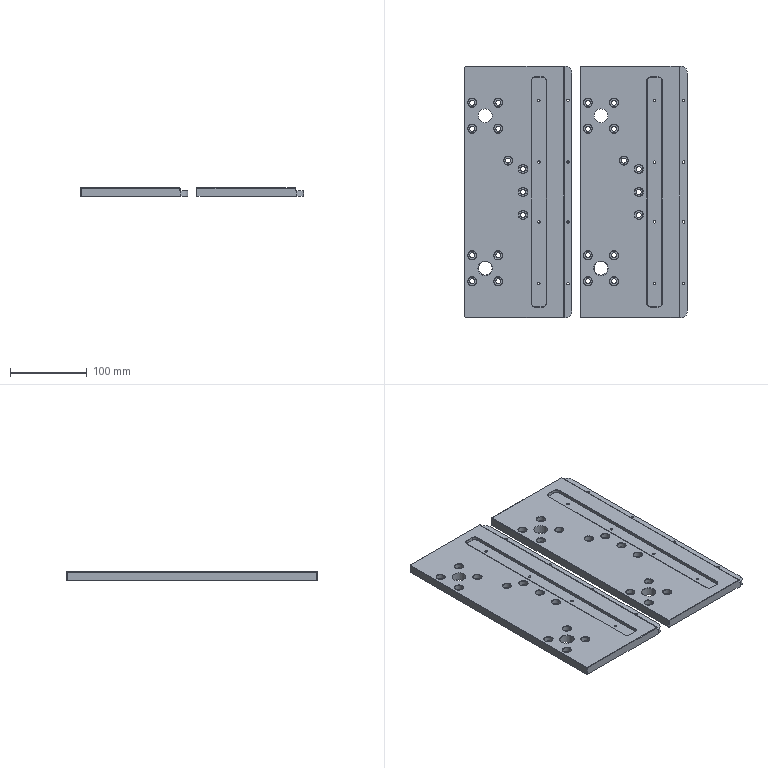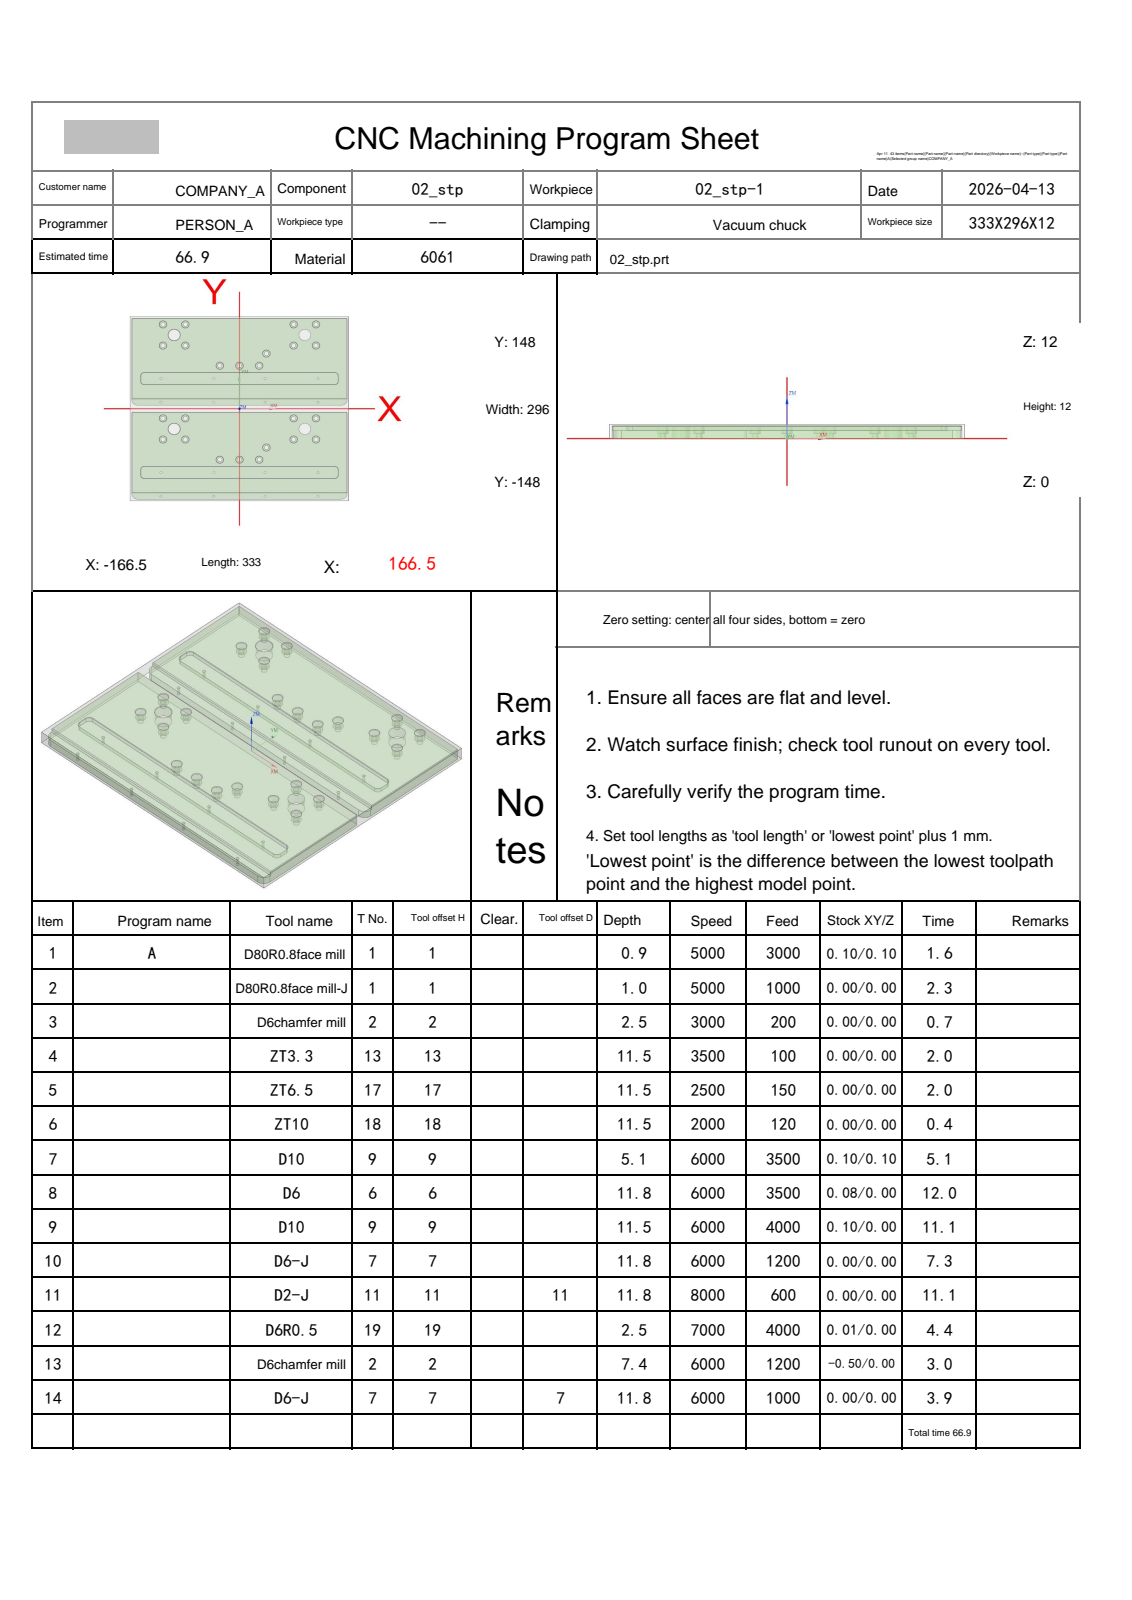NC program | NX | posted by the shop | part box 291 x 328 x 11 mm
Lines 616 to 1679 of 9762:
N8 T06 M06
(D6  D=6. R=0. H=06 ce=0.10 di=0.10)
G00 G90 G54 X-37.711 Y-143.4 M03 S6000
G43 H06 Z31.
M08
Z11.5
G01 X0.0 Z10.513 F3500.
X155.
G03 X159.957 Y-141.3 I0.0 J6.9
G01 X-159.957
G03 X-155. Y-143.4 I4.957 J4.8
G01 X0.0
Y-146.1
X155.
G03 X164.367 Y-138.6 I0.0 J9.6
G01 X-164.367
G03 X-155. Y-146.1 I9.367 J2.1
G01 X0.0
X.5
Z11.013
G00 Z11.5
X-37.711 Y-143.4
Z11.013
G01 X0.0 Z10.025
X155.
G03 X159.957 Y-141.3 I0.0 J6.9
G01 X-159.957
G03 X-155. Y-143.4 I4.957 J4.8
G01 X0.0
Y-146.1
X155.
G03 X164.367 Y-138.6 I0.0 J9.6
G01 X-164.367
G03 X-155. Y-146.1 I9.367 J2.1
G01 X0.0
X.5
Z10.525
G00 Z11.013
X-37.711 Y-143.4
Z10.525
G01 X0.0 Z9.538
X155.
G03 X159.957 Y-141.3 I0.0 J6.9
G01 X-159.957
G03 X-155. Y-143.4 I4.957 J4.8
G01 X0.0
Y-146.1
X155.
G03 X164.367 Y-138.6 I0.0 J9.6
G01 X-164.367
G03 X-155. Y-146.1 I9.367 J2.1
G01 X0.0
X.5
Z10.038
G00 Z10.525
X-37.711 Y-143.4
Z10.038
G01 X0.0 Z9.05
X155.
G03 X159.957 Y-141.3 I0.0 J6.9
G01 X-159.957
G03 X-155. Y-143.4 I4.957 J4.8
G01 X0.0
Y-146.1
X155.
G03 X164.367 Y-138.6 I0.0 J9.6
G01 X-164.367
G03 X-155. Y-146.1 I9.367 J2.1
G01 X0.0
X.5
Z9.55
G00 Z10.038
X-37.711 Y-143.4
Z9.55
G01 X0.0 Z8.563
X155.
G03 X159.957 Y-141.3 I0.0 J6.9
G01 X-159.957
G03 X-155. Y-143.4 I4.957 J4.8
G01 X0.0
Y-146.1
X155.
G03 X164.367 Y-138.6 I0.0 J9.6
G01 X-164.367
G03 X-155. Y-146.1 I9.367 J2.1
G01 X0.0
X.5
Z9.063
G00 Z9.55
X-37.711 Y-143.4
Z9.063
G01 X0.0 Z8.075
X155.
G03 X159.957 Y-141.3 I0.0 J6.9
G01 X-159.957
G03 X-155. Y-143.4 I4.957 J4.8
G01 X0.0
Y-146.1
X155.
G03 X164.367 Y-138.6 I0.0 J9.6
G01 X-164.367
G03 X-155. Y-146.1 I9.367 J2.1
G01 X0.0
X.5
Z8.575
G00 Z9.063
X-37.711 Y-143.4
Z8.575
G01 X0.0 Z7.588
X155.
G03 X159.957 Y-141.3 I0.0 J6.9
G01 X-159.957
G03 X-155. Y-143.4 I4.957 J4.8
G01 X0.0
Y-146.1
X155.
G03 X164.367 Y-138.6 I0.0 J9.6
G01 X-164.367
G03 X-155. Y-146.1 I9.367 J2.1
G01 X0.0
X.5
Z8.088
G00 Z8.575
X-37.711 Y-143.4
Z8.088
G01 X0.0 Z7.1
X155.
G03 X159.957 Y-141.3 I0.0 J6.9
G01 X-159.957
G03 X-155. Y-143.4 I4.957 J4.8
G01 X0.0
Y-146.1
X155.
G03 X164.367 Y-138.6 I0.0 J9.6
G01 X-164.367
G03 X-155. Y-146.1 I9.367 J2.1
G01 X0.0
X.5
Z7.6
G00 Z31.
X-37.711 Y7.6
Z11.5
G01 X0.0 Z10.513
X155.
G03 X159.957 Y9.7 I0.0 J6.9
G01 X-159.957
G03 X-155. Y7.6 I4.957 J4.8
G01 X0.0
Y4.9
X155.
G03 X164.367 Y12.4 I0.0 J9.6
G01 X-164.367
G03 X-155. Y4.9 I9.367 J2.1
G01 X0.0
X.5
Z11.013
G00 Z11.5
X-37.711 Y7.6
Z11.013
G01 X0.0 Z10.025
X155.
G03 X159.957 Y9.7 I0.0 J6.9
G01 X-159.957
G03 X-155. Y7.6 I4.957 J4.8
G01 X0.0
Y4.9
X155.
G03 X164.367 Y12.4 I0.0 J9.6
G01 X-164.367
G03 X-155. Y4.9 I9.367 J2.1
G01 X0.0
X.5
Z10.525
G00 Z11.013
X-37.711 Y7.6
Z10.525
G01 X0.0 Z9.538
X155.
G03 X159.957 Y9.7 I0.0 J6.9
G01 X-159.957
G03 X-155. Y7.6 I4.957 J4.8
G01 X0.0
Y4.9
X155.
G03 X164.367 Y12.4 I0.0 J9.6
G01 X-164.367
G03 X-155. Y4.9 I9.367 J2.1
G01 X0.0
X.5
Z10.038
G00 Z10.525
X-37.711 Y7.6
Z10.038
G01 X0.0 Z9.05
X155.
G03 X159.957 Y9.7 I0.0 J6.9
G01 X-159.957
G03 X-155. Y7.6 I4.957 J4.8
G01 X0.0
Y4.9
X155.
G03 X164.367 Y12.4 I0.0 J9.6
G01 X-164.367
G03 X-155. Y4.9 I9.367 J2.1
G01 X0.0
X.5
Z9.55
G00 Z10.038
X-37.711 Y7.6
Z9.55
G01 X0.0 Z8.563
X155.
G03 X159.957 Y9.7 I0.0 J6.9
G01 X-159.957
G03 X-155. Y7.6 I4.957 J4.8
G01 X0.0
Y4.9
X155.
G03 X164.367 Y12.4 I0.0 J9.6
G01 X-164.367
G03 X-155. Y4.9 I9.367 J2.1
G01 X0.0
X.5
Z9.063
G00 Z9.55
X-37.711 Y7.6
Z9.063
G01 X0.0 Z8.075
X155.
G03 X159.957 Y9.7 I0.0 J6.9
G01 X-159.957
G03 X-155. Y7.6 I4.957 J4.8
G01 X0.0
Y4.9
X155.
G03 X164.367 Y12.4 I0.0 J9.6
G01 X-164.367
G03 X-155. Y4.9 I9.367 J2.1
G01 X0.0
X.5
Z8.575
G00 Z9.063
X-37.711 Y7.6
Z8.575
G01 X0.0 Z7.588
X155.
G03 X159.957 Y9.7 I0.0 J6.9
G01 X-159.957
G03 X-155. Y7.6 I4.957 J4.8
G01 X0.0
Y4.9
X155.
G03 X164.367 Y12.4 I0.0 J9.6
G01 X-164.367
G03 X-155. Y4.9 I9.367 J2.1
G01 X0.0
X.5
Z8.088
G00 Z8.575
X-37.711 Y7.6
Z8.088
G01 X0.0 Z7.1
X155.
G03 X159.957 Y9.7 I0.0 J6.9
G01 X-159.957
G03 X-155. Y7.6 I4.957 J4.8
G01 X0.0
Y4.9
X155.
G03 X164.367 Y12.4 I0.0 J9.6
G01 X-164.367
G03 X-155. Y4.9 I9.367 J2.1
G01 X0.0
X.5
Z7.6
G00 Z31.
G00 G90 X41. Y-62.4 M03 S6000
Z31.
Z11.8
G41 D06
G01 X40.9 Y-62.408 F2000.
G03 X39.802 Y-63.602 I.1 J-1.194
X41. Y-64.8 I1.198 J0.0
X41. Y-64.8 Z11.3 I0.0 J2.4
X41. Y-64.8 Z10.8 I0.0 J2.4
X41. Y-64.8 Z10.3 I0.0 J2.4
X41. Y-64.8 Z9.8 I0.0 J2.4
X41. Y-64.8 Z9.3 I0.0 J2.4
X41. Y-64.8 Z8.8 I0.0 J2.4
X41. Y-64.8 Z8.3 I0.0 J2.4
X41. Y-64.8 Z7.8 I0.0 J2.4
X41. Y-64.8 Z7.3 I0.0 J2.4
X41. Y-64.8 Z6.8 I0.0 J2.4
X41. Y-64.8 Z6.3 I0.0 J2.4
X41. Y-64.8 Z5.8 I0.0 J2.4
X41. Y-64.8 Z5.3 I0.0 J2.4
X41. Y-64.8 Z4.8 I0.0 J2.4
X39.589 Y-60.458 Z4.5 I0.0 J2.4
X38.6 Y-62.4 I1.411 J-1.942
X41. Y-64.8 I2.4 J0.0
X43.4 Y-62.4 I0.0 J2.4
X41. Y-60. I-2.4 J0.0
X39.589 Y-60.458 I0.0 J-2.4
X39.096 Y-61.427 I.704 J-.969
X40.293 Y-62.625 I1.198 J0.0
X40.914 Y-62.452 I0.0 J1.198
G01 G40 X41. Y-62.4
G00 Z31.
X82.5 Y-15.5
Z11.8
G41 D06
G01 X82.4 Y-15.508
G03 X81.302 Y-16.702 I.1 J-1.194
X82.5 Y-17.9 I1.198 J0.0
X82.5 Y-17.9 Z11.3 I0.0 J2.4
X82.5 Y-17.9 Z10.8 I0.0 J2.4
X82.5 Y-17.9 Z10.3 I0.0 J2.4
X82.5 Y-17.9 Z9.8 I0.0 J2.4
X82.5 Y-17.9 Z9.3 I0.0 J2.4
X82.5 Y-17.9 Z8.8 I0.0 J2.4
X82.5 Y-17.9 Z8.3 I0.0 J2.4
X82.5 Y-17.9 Z7.8 I0.0 J2.4
X82.5 Y-17.9 Z7.3 I0.0 J2.4
X82.5 Y-17.9 Z6.8 I0.0 J2.4
X82.5 Y-17.9 Z6.3 I0.0 J2.4
X82.5 Y-17.9 Z5.8 I0.0 J2.4
X82.5 Y-17.9 Z5.3 I0.0 J2.4
X82.5 Y-17.9 Z4.8 I0.0 J2.4
X81.089 Y-13.558 Z4.5 I0.0 J2.4
X80.1 Y-15.5 I1.411 J-1.942
X82.5 Y-17.9 I2.4 J0.0
X84.9 Y-15.5 I0.0 J2.4
X82.5 Y-13.1 I-2.4 J0.0
X81.089 Y-13.558 I0.0 J-2.4
X80.596 Y-14.527 I.704 J-.969
X81.793 Y-15.725 I1.198 J0.0
X82.414 Y-15.552 I0.0 J1.198
G01 G40 X82.5 Y-15.5
G00 Z31.
X116.5
Z11.8
G41 D06
G01 X116.4 Y-15.508
G03 X115.302 Y-16.702 I.1 J-1.194
X116.5 Y-17.9 I1.198 J0.0
X116.5 Y-17.9 Z11.3 I0.0 J2.4
X116.5 Y-17.9 Z10.8 I0.0 J2.4
X116.5 Y-17.9 Z10.3 I0.0 J2.4
X116.5 Y-17.9 Z9.8 I0.0 J2.4
X116.5 Y-17.9 Z9.3 I0.0 J2.4
X116.5 Y-17.9 Z8.8 I0.0 J2.4
X116.5 Y-17.9 Z8.3 I0.0 J2.4
X116.5 Y-17.9 Z7.8 I0.0 J2.4
X116.5 Y-17.9 Z7.3 I0.0 J2.4
X116.5 Y-17.9 Z6.8 I0.0 J2.4
X116.5 Y-17.9 Z6.3 I0.0 J2.4
X116.5 Y-17.9 Z5.8 I0.0 J2.4
X116.5 Y-17.9 Z5.3 I0.0 J2.4
X116.5 Y-17.9 Z4.8 I0.0 J2.4
X115.089 Y-13.558 Z4.5 I0.0 J2.4
X114.1 Y-15.5 I1.411 J-1.942
X116.5 Y-17.9 I2.4 J0.0
X118.9 Y-15.5 I0.0 J2.4
X116.5 Y-13.1 I-2.4 J0.0
X115.089 Y-13.558 I0.0 J-2.4
X114.596 Y-14.527 I.704 J-.969
X115.793 Y-15.725 I1.198 J0.0
X116.414 Y-15.552 I0.0 J1.198
G01 G40 X116.5 Y-15.5
G00 Z31.
Y-49.5
Z11.8
G41 D06
G01 X116.4 Y-49.508
G03 X115.302 Y-50.702 I.1 J-1.194
X116.5 Y-51.9 I1.198 J0.0
X116.5 Y-51.9 Z11.3 I0.0 J2.4
X116.5 Y-51.9 Z10.8 I0.0 J2.4
X116.5 Y-51.9 Z10.3 I0.0 J2.4
X116.5 Y-51.9 Z9.8 I0.0 J2.4
X116.5 Y-51.9 Z9.3 I0.0 J2.4
X116.5 Y-51.9 Z8.8 I0.0 J2.4
X116.5 Y-51.9 Z8.3 I0.0 J2.4
X116.5 Y-51.9 Z7.8 I0.0 J2.4
X116.5 Y-51.9 Z7.3 I0.0 J2.4
X116.5 Y-51.9 Z6.8 I0.0 J2.4
X116.5 Y-51.9 Z6.3 I0.0 J2.4
X116.5 Y-51.9 Z5.8 I0.0 J2.4
X116.5 Y-51.9 Z5.3 I0.0 J2.4
X116.5 Y-51.9 Z4.8 I0.0 J2.4
X115.089 Y-47.558 Z4.5 I0.0 J2.4
X114.1 Y-49.5 I1.411 J-1.942
X116.5 Y-51.9 I2.4 J0.0
X118.9 Y-49.5 I0.0 J2.4
X116.5 Y-47.1 I-2.4 J0.0
X115.089 Y-47.558 I0.0 J-2.4
X114.596 Y-48.527 I.704 J-.969
X115.793 Y-49.725 I1.198 J0.0
X116.414 Y-49.552 I0.0 J1.198
G01 G40 X116.5 Y-49.5
G00 Z31.
X82.5
Z11.8
G41 D06
G01 X82.4 Y-49.508
G03 X81.302 Y-50.702 I.1 J-1.194
X82.5 Y-51.9 I1.198 J0.0
X82.5 Y-51.9 Z11.3 I0.0 J2.4
X82.5 Y-51.9 Z10.8 I0.0 J2.4
X82.5 Y-51.9 Z10.3 I0.0 J2.4
X82.5 Y-51.9 Z9.8 I0.0 J2.4
X82.5 Y-51.9 Z9.3 I0.0 J2.4
X82.5 Y-51.9 Z8.8 I0.0 J2.4
X82.5 Y-51.9 Z8.3 I0.0 J2.4
X82.5 Y-51.9 Z7.8 I0.0 J2.4
X82.5 Y-51.9 Z7.3 I0.0 J2.4
X82.5 Y-51.9 Z6.8 I0.0 J2.4
X82.5 Y-51.9 Z6.3 I0.0 J2.4
X82.5 Y-51.9 Z5.8 I0.0 J2.4
X82.5 Y-51.9 Z5.3 I0.0 J2.4
X82.5 Y-51.9 Z4.8 I0.0 J2.4
X81.089 Y-47.558 Z4.5 I0.0 J2.4
X80.1 Y-49.5 I1.411 J-1.942
X82.5 Y-51.9 I2.4 J0.0
X84.9 Y-49.5 I0.0 J2.4
X82.5 Y-47.1 I-2.4 J0.0
X81.089 Y-47.558 I0.0 J-2.4
X80.596 Y-48.527 I.704 J-.969
X81.793 Y-49.725 I1.198 J0.0
X82.414 Y-49.552 I0.0 J1.198
G01 G40 X82.5 Y-49.5
G00 Z31.
X30.05 Y-81.9
Z11.8
G41 D06
G01 X29.95 Y-81.908
G03 X28.852 Y-83.102 I.1 J-1.194
X30.05 Y-84.3 I1.198 J0.0
X30.05 Y-84.3 Z11.3 I0.0 J2.4
X30.05 Y-84.3 Z10.8 I0.0 J2.4
X30.05 Y-84.3 Z10.3 I0.0 J2.4
X30.05 Y-84.3 Z9.8 I0.0 J2.4
X30.05 Y-84.3 Z9.3 I0.0 J2.4
X30.05 Y-84.3 Z8.8 I0.0 J2.4
X30.05 Y-84.3 Z8.3 I0.0 J2.4
X30.05 Y-84.3 Z7.8 I0.0 J2.4
X30.05 Y-84.3 Z7.3 I0.0 J2.4
X30.05 Y-84.3 Z6.8 I0.0 J2.4
X30.05 Y-84.3 Z6.3 I0.0 J2.4
X30.05 Y-84.3 Z5.8 I0.0 J2.4
X30.05 Y-84.3 Z5.3 I0.0 J2.4
X30.05 Y-84.3 Z4.8 I0.0 J2.4
X28.639 Y-79.958 Z4.5 I0.0 J2.4
X27.65 Y-81.9 I1.411 J-1.942
X30.05 Y-84.3 I2.4 J0.0
X32.45 Y-81.9 I0.0 J2.4
X30.05 Y-79.5 I-2.4 J0.0
X28.639 Y-79.958 I0.0 J-2.4
X28.146 Y-80.927 I.704 J-.969
X29.343 Y-82.125 I1.198 J0.0
X29.964 Y-81.952 I0.0 J1.198
G01 G40 X30.05 Y-81.9
G00 Z31.
X.05
Z11.8
G41 D06
G01 X-.05 Y-81.908
G03 X-1.148 Y-83.102 I.1 J-1.194
X.05 Y-84.3 I1.198 J0.0
X.05 Y-84.3 Z11.3 I0.0 J2.4
X.05 Y-84.3 Z10.8 I0.0 J2.4
X.05 Y-84.3 Z10.3 I0.0 J2.4
X.05 Y-84.3 Z9.8 I0.0 J2.4
X.05 Y-84.3 Z9.3 I0.0 J2.4
X.05 Y-84.3 Z8.8 I0.0 J2.4
X.05 Y-84.3 Z8.3 I0.0 J2.4
X.05 Y-84.3 Z7.8 I0.0 J2.4
X.05 Y-84.3 Z7.3 I0.0 J2.4
X.05 Y-84.3 Z6.8 I0.0 J2.4
X.05 Y-84.3 Z6.3 I0.0 J2.4
X.05 Y-84.3 Z5.8 I0.0 J2.4
X.05 Y-84.3 Z5.3 I0.0 J2.4
X.05 Y-84.3 Z4.8 I0.0 J2.4
X-1.361 Y-79.958 Z4.5 I0.0 J2.4
X-2.35 Y-81.9 I1.411 J-1.942
X.05 Y-84.3 I2.4 J0.0
X2.45 Y-81.9 I0.0 J2.4
X.05 Y-79.5 I-2.4 J0.0
X-1.361 Y-79.958 I0.0 J-2.4
X-1.854 Y-80.927 I.704 J-.969
X-.657 Y-82.125 I1.198 J0.0
X-.036 Y-81.952 I0.0 J1.198
G01 G40 X.05 Y-81.9
G00 Z31.
X-29.95
Z11.8
G41 D06
G01 X-30.05 Y-81.908
G03 X-31.148 Y-83.102 I.1 J-1.194
X-29.95 Y-84.3 I1.198 J0.0
X-29.95 Y-84.3 Z11.3 I0.0 J2.4
X-29.95 Y-84.3 Z10.8 I0.0 J2.4
X-29.95 Y-84.3 Z10.3 I0.0 J2.4
X-29.95 Y-84.3 Z9.8 I0.0 J2.4
X-29.95 Y-84.3 Z9.3 I0.0 J2.4
X-29.95 Y-84.3 Z8.8 I0.0 J2.4
X-29.95 Y-84.3 Z8.3 I0.0 J2.4
X-29.95 Y-84.3 Z7.8 I0.0 J2.4
X-29.95 Y-84.3 Z7.3 I0.0 J2.4
X-29.95 Y-84.3 Z6.8 I0.0 J2.4
X-29.95 Y-84.3 Z6.3 I0.0 J2.4
X-29.95 Y-84.3 Z5.8 I0.0 J2.4
X-29.95 Y-84.3 Z5.3 I0.0 J2.4
X-29.95 Y-84.3 Z4.8 I0.0 J2.4
X-31.361 Y-79.958 Z4.5 I0.0 J2.4
X-32.35 Y-81.9 I1.411 J-1.942
X-29.95 Y-84.3 I2.4 J0.0
X-27.55 Y-81.9 I0.0 J2.4
X-29.95 Y-79.5 I-2.4 J0.0
X-31.361 Y-79.958 I0.0 J-2.4
X-31.854 Y-80.927 I.704 J-.969
X-30.657 Y-82.125 I1.198 J0.0
X-30.036 Y-81.952 I0.0 J1.198
G01 G40 X-29.95 Y-81.9
G00 Z31.
X-82.5 Y-49.5
Z11.8
G41 D06
G01 X-82.6 Y-49.508
G03 X-83.698 Y-50.702 I.1 J-1.194
X-82.5 Y-51.9 I1.198 J0.0
X-82.5 Y-51.9 Z11.3 I0.0 J2.4
X-82.5 Y-51.9 Z10.8 I0.0 J2.4
X-82.5 Y-51.9 Z10.3 I0.0 J2.4
X-82.5 Y-51.9 Z9.8 I0.0 J2.4
X-82.5 Y-51.9 Z9.3 I0.0 J2.4
X-82.5 Y-51.9 Z8.8 I0.0 J2.4
X-82.5 Y-51.9 Z8.3 I0.0 J2.4
X-82.5 Y-51.9 Z7.8 I0.0 J2.4
X-82.5 Y-51.9 Z7.3 I0.0 J2.4
X-82.5 Y-51.9 Z6.8 I0.0 J2.4
X-82.5 Y-51.9 Z6.3 I0.0 J2.4
X-82.5 Y-51.9 Z5.8 I0.0 J2.4
X-82.5 Y-51.9 Z5.3 I0.0 J2.4
X-82.5 Y-51.9 Z4.8 I0.0 J2.4
X-83.911 Y-47.558 Z4.5 I0.0 J2.4
X-84.9 Y-49.5 I1.411 J-1.942
X-82.5 Y-51.9 I2.4 J0.0
X-80.1 Y-49.5 I0.0 J2.4
X-82.5 Y-47.1 I-2.4 J0.0
X-83.911 Y-47.558 I0.0 J-2.4
X-84.404 Y-48.527 I.704 J-.969
X-83.207 Y-49.725 I1.198 J0.0
X-82.586 Y-49.552 I0.0 J1.198
G01 G40 X-82.5 Y-49.5
G00 Z31.
X-116.5
Z11.8
G41 D06
G01 X-116.6 Y-49.508
G03 X-117.698 Y-50.702 I.1 J-1.194
X-116.5 Y-51.9 I1.198 J0.0
X-116.5 Y-51.9 Z11.3 I0.0 J2.4
X-116.5 Y-51.9 Z10.8 I0.0 J2.4
X-116.5 Y-51.9 Z10.3 I0.0 J2.4
X-116.5 Y-51.9 Z9.8 I0.0 J2.4
X-116.5 Y-51.9 Z9.3 I0.0 J2.4
X-116.5 Y-51.9 Z8.8 I0.0 J2.4
X-116.5 Y-51.9 Z8.3 I0.0 J2.4
X-116.5 Y-51.9 Z7.8 I0.0 J2.4
X-116.5 Y-51.9 Z7.3 I0.0 J2.4
X-116.5 Y-51.9 Z6.8 I0.0 J2.4
X-116.5 Y-51.9 Z6.3 I0.0 J2.4
X-116.5 Y-51.9 Z5.8 I0.0 J2.4
X-116.5 Y-51.9 Z5.3 I0.0 J2.4
X-116.5 Y-51.9 Z4.8 I0.0 J2.4
X-117.911 Y-47.558 Z4.5 I0.0 J2.4
X-118.9 Y-49.5 I1.411 J-1.942
X-116.5 Y-51.9 I2.4 J0.0
X-114.1 Y-49.5 I0.0 J2.4
X-116.5 Y-47.1 I-2.4 J0.0
X-117.911 Y-47.558 I0.0 J-2.4
X-118.404 Y-48.527 I.704 J-.969
X-117.207 Y-49.725 I1.198 J0.0
X-116.586 Y-49.552 I0.0 J1.198
G01 G40 X-116.5 Y-49.5
G00 Z31.
Y-15.5
Z11.8
G41 D06
G01 X-116.6 Y-15.508
G03 X-117.698 Y-16.702 I.1 J-1.194
X-116.5 Y-17.9 I1.198 J0.0
X-116.5 Y-17.9 Z11.3 I0.0 J2.4
X-116.5 Y-17.9 Z10.8 I0.0 J2.4
X-116.5 Y-17.9 Z10.3 I0.0 J2.4
X-116.5 Y-17.9 Z9.8 I0.0 J2.4
X-116.5 Y-17.9 Z9.3 I0.0 J2.4
X-116.5 Y-17.9 Z8.8 I0.0 J2.4
X-116.5 Y-17.9 Z8.3 I0.0 J2.4
X-116.5 Y-17.9 Z7.8 I0.0 J2.4
X-116.5 Y-17.9 Z7.3 I0.0 J2.4
X-116.5 Y-17.9 Z6.8 I0.0 J2.4
X-116.5 Y-17.9 Z6.3 I0.0 J2.4
X-116.5 Y-17.9 Z5.8 I0.0 J2.4
X-116.5 Y-17.9 Z5.3 I0.0 J2.4
X-116.5 Y-17.9 Z4.8 I0.0 J2.4
X-117.911 Y-13.558 Z4.5 I0.0 J2.4
X-118.9 Y-15.5 I1.411 J-1.942
X-116.5 Y-17.9 I2.4 J0.0
X-114.1 Y-15.5 I0.0 J2.4
X-116.5 Y-13.1 I-2.4 J0.0
X-117.911 Y-13.558 I0.0 J-2.4
X-118.404 Y-14.527 I.704 J-.969
X-117.207 Y-15.725 I1.198 J0.0
X-116.586 Y-15.552 I0.0 J1.198
G01 G40 X-116.5 Y-15.5
G00 Z31.
X-82.5
Z11.8
G41 D06
G01 X-82.6 Y-15.508
G03 X-83.698 Y-16.702 I.1 J-1.194
X-82.5 Y-17.9 I1.198 J0.0
X-82.5 Y-17.9 Z11.3 I0.0 J2.4
X-82.5 Y-17.9 Z10.8 I0.0 J2.4
X-82.5 Y-17.9 Z10.3 I0.0 J2.4
X-82.5 Y-17.9 Z9.8 I0.0 J2.4
X-82.5 Y-17.9 Z9.3 I0.0 J2.4
X-82.5 Y-17.9 Z8.8 I0.0 J2.4
X-82.5 Y-17.9 Z8.3 I0.0 J2.4
X-82.5 Y-17.9 Z7.8 I0.0 J2.4
X-82.5 Y-17.9 Z7.3 I0.0 J2.4
X-82.5 Y-17.9 Z6.8 I0.0 J2.4
X-82.5 Y-17.9 Z6.3 I0.0 J2.4
X-82.5 Y-17.9 Z5.8 I0.0 J2.4
X-82.5 Y-17.9 Z5.3 I0.0 J2.4
X-82.5 Y-17.9 Z4.8 I0.0 J2.4
X-83.911 Y-13.558 Z4.5 I0.0 J2.4
X-84.9 Y-15.5 I1.411 J-1.942
X-82.5 Y-17.9 I2.4 J0.0
X-80.1 Y-15.5 I0.0 J2.4
X-82.5 Y-13.1 I-2.4 J0.0
X-83.911 Y-13.558 I0.0 J-2.4
X-84.404 Y-14.527 I.704 J-.969
X-83.207 Y-15.725 I1.198 J0.0
X-82.586 Y-15.552 I0.0 J1.198
G01 G40 X-82.5 Y-15.5
G00 Z31.
X-116.5 Y101.5
Z11.8
G41 D06
G01 X-116.6 Y101.492
G03 X-117.698 Y100.298 I.1 J-1.194
X-116.5 Y99.1 I1.198 J0.0
X-116.5 Y99.1 Z11.3 I0.0 J2.4
X-116.5 Y99.1 Z10.8 I0.0 J2.4
X-116.5 Y99.1 Z10.3 I0.0 J2.4
X-116.5 Y99.1 Z9.8 I0.0 J2.4
X-116.5 Y99.1 Z9.3 I0.0 J2.4
X-116.5 Y99.1 Z8.8 I0.0 J2.4
X-116.5 Y99.1 Z8.3 I0.0 J2.4
X-116.5 Y99.1 Z7.8 I0.0 J2.4
X-116.5 Y99.1 Z7.3 I0.0 J2.4
X-116.5 Y99.1 Z6.8 I0.0 J2.4
X-116.5 Y99.1 Z6.3 I0.0 J2.4
X-116.5 Y99.1 Z5.8 I0.0 J2.4
X-116.5 Y99.1 Z5.3 I0.0 J2.4
X-116.5 Y99.1 Z4.8 I0.0 J2.4
X-117.911 Y103.442 Z4.5 I0.0 J2.4
X-118.9 Y101.5 I1.411 J-1.942
X-116.5 Y99.1 I2.4 J0.0
X-114.1 Y101.5 I0.0 J2.4
X-116.5 Y103.9 I-2.4 J0.0
X-117.911 Y103.442 I0.0 J-2.4
X-118.404 Y102.473 I.704 J-.969
X-117.207 Y101.275 I1.198 J0.0
X-116.586 Y101.448 I0.0 J1.198
G01 G40 X-116.5 Y101.5
G00 Z31.
Y135.5
Z11.8
G41 D06
G01 X-116.6 Y135.492
G03 X-117.698 Y134.298 I.1 J-1.194
X-116.5 Y133.1 I1.198 J0.0
X-116.5 Y133.1 Z11.3 I0.0 J2.4
X-116.5 Y133.1 Z10.8 I0.0 J2.4
X-116.5 Y133.1 Z10.3 I0.0 J2.4
X-116.5 Y133.1 Z9.8 I0.0 J2.4
X-116.5 Y133.1 Z9.3 I0.0 J2.4
X-116.5 Y133.1 Z8.8 I0.0 J2.4
X-116.5 Y133.1 Z8.3 I0.0 J2.4
X-116.5 Y133.1 Z7.8 I0.0 J2.4
X-116.5 Y133.1 Z7.3 I0.0 J2.4
X-116.5 Y133.1 Z6.8 I0.0 J2.4
X-116.5 Y133.1 Z6.3 I0.0 J2.4
X-116.5 Y133.1 Z5.8 I0.0 J2.4
X-116.5 Y133.1 Z5.3 I0.0 J2.4
X-116.5 Y133.1 Z4.8 I0.0 J2.4
X-117.911 Y137.442 Z4.5 I0.0 J2.4
X-118.9 Y135.5 I1.411 J-1.942
X-116.5 Y133.1 I2.4 J0.0
X-114.1 Y135.5 I0.0 J2.4
X-116.5 Y137.9 I-2.4 J0.0
X-117.911 Y137.442 I0.0 J-2.4
X-118.404 Y136.473 I.704 J-.969
X-117.207 Y135.275 I1.198 J0.0
X-116.586 Y135.448 I0.0 J1.198
G01 G40 X-116.5 Y135.5
G00 Z31.
X-82.5
Z11.8
G41 D06
G01 X-82.6 Y135.492
G03 X-83.698 Y134.298 I.1 J-1.194
X-82.5 Y133.1 I1.198 J0.0
X-82.5 Y133.1 Z11.3 I0.0 J2.4
X-82.5 Y133.1 Z10.8 I0.0 J2.4
X-82.5 Y133.1 Z10.3 I0.0 J2.4
X-82.5 Y133.1 Z9.8 I0.0 J2.4
X-82.5 Y133.1 Z9.3 I0.0 J2.4
X-82.5 Y133.1 Z8.8 I0.0 J2.4
X-82.5 Y133.1 Z8.3 I0.0 J2.4
X-82.5 Y133.1 Z7.8 I0.0 J2.4
X-82.5 Y133.1 Z7.3 I0.0 J2.4
X-82.5 Y133.1 Z6.8 I0.0 J2.4
X-82.5 Y133.1 Z6.3 I0.0 J2.4
X-82.5 Y133.1 Z5.8 I0.0 J2.4
X-82.5 Y133.1 Z5.3 I0.0 J2.4
X-82.5 Y133.1 Z4.8 I0.0 J2.4
X-83.911 Y137.442 Z4.5 I0.0 J2.4
X-84.9 Y135.5 I1.411 J-1.942
X-82.5 Y133.1 I2.4 J0.0
X-80.1 Y135.5 I0.0 J2.4
X-82.5 Y137.9 I-2.4 J0.0
X-83.911 Y137.442 I0.0 J-2.4
X-84.404 Y136.473 I.704 J-.969
X-83.207 Y135.275 I1.198 J0.0
X-82.586 Y135.448 I0.0 J1.198
G01 G40 X-82.5 Y135.5
G00 Z31.
Y101.5
Z11.8
G41 D06
G01 X-82.6 Y101.492
G03 X-83.698 Y100.298 I.1 J-1.194
X-82.5 Y99.1 I1.198 J0.0
X-82.5 Y99.1 Z11.3 I0.0 J2.4
X-82.5 Y99.1 Z10.8 I0.0 J2.4
X-82.5 Y99.1 Z10.3 I0.0 J2.4
X-82.5 Y99.1 Z9.8 I0.0 J2.4
X-82.5 Y99.1 Z9.3 I0.0 J2.4
X-82.5 Y99.1 Z8.8 I0.0 J2.4
X-82.5 Y99.1 Z8.3 I0.0 J2.4
X-82.5 Y99.1 Z7.8 I0.0 J2.4
X-82.5 Y99.1 Z7.3 I0.0 J2.4
X-82.5 Y99.1 Z6.8 I0.0 J2.4
X-82.5 Y99.1 Z6.3 I0.0 J2.4
X-82.5 Y99.1 Z5.8 I0.0 J2.4
X-82.5 Y99.1 Z5.3 I0.0 J2.4
X-82.5 Y99.1 Z4.8 I0.0 J2.4
X-83.911 Y103.442 Z4.5 I0.0 J2.4
X-84.9 Y101.5 I1.411 J-1.942
X-82.5 Y99.1 I2.4 J0.0
X-80.1 Y101.5 I0.0 J2.4
X-82.5 Y103.9 I-2.4 J0.0
X-83.911 Y103.442 I0.0 J-2.4
X-84.404 Y102.473 I.704 J-.969
X-83.207 Y101.275 I1.198 J0.0
X-82.586 Y101.448 I0.0 J1.198
G01 G40 X-82.5 Y101.5
G00 Z31.
X-29.95 Y69.1
Z11.8
G41 D06
G01 X-30.05 Y69.092
G03 X-31.148 Y67.898 I.1 J-1.194
X-29.95 Y66.7 I1.198 J0.0
X-29.95 Y66.7 Z11.3 I0.0 J2.4
X-29.95 Y66.7 Z10.8 I0.0 J2.4
X-29.95 Y66.7 Z10.3 I0.0 J2.4
X-29.95 Y66.7 Z9.8 I0.0 J2.4
X-29.95 Y66.7 Z9.3 I0.0 J2.4
X-29.95 Y66.7 Z8.8 I0.0 J2.4
X-29.95 Y66.7 Z8.3 I0.0 J2.4
X-29.95 Y66.7 Z7.8 I0.0 J2.4
X-29.95 Y66.7 Z7.3 I0.0 J2.4
X-29.95 Y66.7 Z6.8 I0.0 J2.4
X-29.95 Y66.7 Z6.3 I0.0 J2.4
X-29.95 Y66.7 Z5.8 I0.0 J2.4
X-29.95 Y66.7 Z5.3 I0.0 J2.4
X-29.95 Y66.7 Z4.8 I0.0 J2.4
X-31.361 Y71.042 Z4.5 I0.0 J2.4
X-32.35 Y69.1 I1.411 J-1.942
X-29.95 Y66.7 I2.4 J0.0
X-27.55 Y69.1 I0.0 J2.4
X-29.95 Y71.5 I-2.4 J0.0
X-31.361 Y71.042 I0.0 J-2.4
X-31.854 Y70.073 I.704 J-.969
X-30.657 Y68.875 I1.198 J0.0
X-30.036 Y69.048 I0.0 J1.198
G01 G40 X-29.95 Y69.1
G00 Z31.
X.05
Z11.8
G41 D06
G01 X-.05 Y69.092
G03 X-1.148 Y67.898 I.1 J-1.194
X.05 Y66.7 I1.198 J0.0
X.05 Y66.7 Z11.3 I0.0 J2.4
X.05 Y66.7 Z10.8 I0.0 J2.4
X.05 Y66.7 Z10.3 I0.0 J2.4
X.05 Y66.7 Z9.8 I0.0 J2.4
X.05 Y66.7 Z9.3 I0.0 J2.4
X.05 Y66.7 Z8.8 I0.0 J2.4
X.05 Y66.7 Z8.3 I0.0 J2.4
X.05 Y66.7 Z7.8 I0.0 J2.4
X.05 Y66.7 Z7.3 I0.0 J2.4
X.05 Y66.7 Z6.8 I0.0 J2.4
X.05 Y66.7 Z6.3 I0.0 J2.4
X.05 Y66.7 Z5.8 I0.0 J2.4
X.05 Y66.7 Z5.3 I0.0 J2.4
X.05 Y66.7 Z4.8 I0.0 J2.4
X-1.361 Y71.042 Z4.5 I0.0 J2.4
X-2.35 Y69.1 I1.411 J-1.942
X.05 Y66.7 I2.4 J0.0
X2.45 Y69.1 I0.0 J2.4
X.05 Y71.5 I-2.4 J0.0
X-1.361 Y71.042 I0.0 J-2.4
X-1.854 Y70.073 I.704 J-.969
X-.657 Y68.875 I1.198 J0.0
X-.036 Y69.048 I0.0 J1.198
G01 G40 X.05 Y69.1
G00 Z31.
X30.05
Z11.8
G41 D06
G01 X29.95 Y69.092
G03 X28.852 Y67.898 I.1 J-1.194
X30.05 Y66.7 I1.198 J0.0
X30.05 Y66.7 Z11.3 I0.0 J2.4
X30.05 Y66.7 Z10.8 I0.0 J2.4
X30.05 Y66.7 Z10.3 I0.0 J2.4
X30.05 Y66.7 Z9.8 I0.0 J2.4
X30.05 Y66.7 Z9.3 I0.0 J2.4
X30.05 Y66.7 Z8.8 I0.0 J2.4
X30.05 Y66.7 Z8.3 I0.0 J2.4
X30.05 Y66.7 Z7.8 I0.0 J2.4
X30.05 Y66.7 Z7.3 I0.0 J2.4
X30.05 Y66.7 Z6.8 I0.0 J2.4
X30.05 Y66.7 Z6.3 I0.0 J2.4
X30.05 Y66.7 Z5.8 I0.0 J2.4
X30.05 Y66.7 Z5.3 I0.0 J2.4
X30.05 Y66.7 Z4.8 I0.0 J2.4
X28.639 Y71.042 Z4.5 I0.0 J2.4
X27.65 Y69.1 I1.411 J-1.942
X30.05 Y66.7 I2.4 J0.0
X32.45 Y69.1 I0.0 J2.4
X30.05 Y71.5 I-2.4 J0.0
X28.639 Y71.042 I0.0 J-2.4
X28.146 Y70.073 I.704 J-.969
X29.343 Y68.875 I1.198 J0.0
X29.964 Y69.048 I0.0 J1.198
G01 G40 X30.05 Y69.1
G00 Z31.
X41. Y88.6
Z11.8
G41 D06
G01 X40.9 Y88.592
G03 X39.802 Y87.398 I.1 J-1.194
X41. Y86.2 I1.198 J0.0
X41. Y86.2 Z11.3 I0.0 J2.4
X41. Y86.2 Z10.8 I0.0 J2.4
X41. Y86.2 Z10.3 I0.0 J2.4
X41. Y86.2 Z9.8 I0.0 J2.4
X41. Y86.2 Z9.3 I0.0 J2.4
X41. Y86.2 Z8.8 I0.0 J2.4
X41. Y86.2 Z8.3 I0.0 J2.4
X41. Y86.2 Z7.8 I0.0 J2.4
X41. Y86.2 Z7.3 I0.0 J2.4
X41. Y86.2 Z6.8 I0.0 J2.4
X41. Y86.2 Z6.3 I0.0 J2.4
X41. Y86.2 Z5.8 I0.0 J2.4
X41. Y86.2 Z5.3 I0.0 J2.4
X41. Y86.2 Z4.8 I0.0 J2.4
X39.589 Y90.542 Z4.5 I0.0 J2.4
X38.6 Y88.6 I1.411 J-1.942
X41. Y86.2 I2.4 J0.0
X43.4 Y88.6 I0.0 J2.4
X41. Y91. I-2.4 J0.0
X39.589 Y90.542 I0.0 J-2.4
X39.096 Y89.573 I.704 J-.969
X40.293 Y88.375 I1.198 J0.0
X40.914 Y88.548 I0.0 J1.198
G01 G40 X41. Y88.6
G00 Z31.
X82.5 Y101.5
Z11.8
G41 D06
G01 X82.4 Y101.492
G03 X81.302 Y100.298 I.1 J-1.194
X82.5 Y99.1 I1.198 J0.0
X82.5 Y99.1 Z11.3 I0.0 J2.4
X82.5 Y99.1 Z10.8 I0.0 J2.4
X82.5 Y99.1 Z10.3 I0.0 J2.4
X82.5 Y99.1 Z9.8 I0.0 J2.4
X82.5 Y99.1 Z9.3 I0.0 J2.4
X82.5 Y99.1 Z8.8 I0.0 J2.4
X82.5 Y99.1 Z8.3 I0.0 J2.4
X82.5 Y99.1 Z7.8 I0.0 J2.4
X82.5 Y99.1 Z7.3 I0.0 J2.4
X82.5 Y99.1 Z6.8 I0.0 J2.4
X82.5 Y99.1 Z6.3 I0.0 J2.4
X82.5 Y99.1 Z5.8 I0.0 J2.4
X82.5 Y99.1 Z5.3 I0.0 J2.4
X82.5 Y99.1 Z4.8 I0.0 J2.4
X81.089 Y103.442 Z4.5 I0.0 J2.4
X80.1 Y101.5 I1.411 J-1.942
X82.5 Y99.1 I2.4 J0.0
X84.9 Y101.5 I0.0 J2.4
X82.5 Y103.9 I-2.4 J0.0
X81.089 Y103.442 I0.0 J-2.4
X80.596 Y102.473 I.704 J-.969
X81.793 Y101.275 I1.198 J0.0
X82.414 Y101.448 I0.0 J1.198
G01 G40 X82.5 Y101.5
G00 Z31.
Y135.5
Z11.8
G41 D06
G01 X82.4 Y135.492
G03 X81.302 Y134.298 I.1 J-1.194
X82.5 Y133.1 I1.198 J0.0
X82.5 Y133.1 Z11.3 I0.0 J2.4
X82.5 Y133.1 Z10.8 I0.0 J2.4
X82.5 Y133.1 Z10.3 I0.0 J2.4
X82.5 Y133.1 Z9.8 I0.0 J2.4
X82.5 Y133.1 Z9.3 I0.0 J2.4
X82.5 Y133.1 Z8.8 I0.0 J2.4
X82.5 Y133.1 Z8.3 I0.0 J2.4
X82.5 Y133.1 Z7.8 I0.0 J2.4
X82.5 Y133.1 Z7.3 I0.0 J2.4
X82.5 Y133.1 Z6.8 I0.0 J2.4
X82.5 Y133.1 Z6.3 I0.0 J2.4
X82.5 Y133.1 Z5.8 I0.0 J2.4
X82.5 Y133.1 Z5.3 I0.0 J2.4
X82.5 Y133.1 Z4.8 I0.0 J2.4
X81.089 Y137.442 Z4.5 I0.0 J2.4
X80.1 Y135.5 I1.411 J-1.942
X82.5 Y133.1 I2.4 J0.0
X84.9 Y135.5 I0.0 J2.4
X82.5 Y137.9 I-2.4 J0.0
X81.089 Y137.442 I0.0 J-2.4
X80.596 Y136.473 I.704 J-.969
X81.793 Y135.275 I1.198 J0.0
X82.414 Y135.448 I0.0 J1.198
G01 G40 X82.5 Y135.5
G00 Z31.
X116.5
Z11.8
G41 D06
G01 X116.4 Y135.492
G03 X115.302 Y134.298 I.1 J-1.194
X116.5 Y133.1 I1.198 J0.0
X116.5 Y133.1 Z11.3 I0.0 J2.4
X116.5 Y133.1 Z10.8 I0.0 J2.4
X116.5 Y133.1 Z10.3 I0.0 J2.4
X116.5 Y133.1 Z9.8 I0.0 J2.4
X116.5 Y133.1 Z9.3 I0.0 J2.4
X116.5 Y133.1 Z8.8 I0.0 J2.4
X116.5 Y133.1 Z8.3 I0.0 J2.4
X116.5 Y133.1 Z7.8 I0.0 J2.4
X116.5 Y133.1 Z7.3 I0.0 J2.4
X116.5 Y133.1 Z6.8 I0.0 J2.4
X116.5 Y133.1 Z6.3 I0.0 J2.4
X116.5 Y133.1 Z5.8 I0.0 J2.4
X116.5 Y133.1 Z5.3 I0.0 J2.4
X116.5 Y133.1 Z4.8 I0.0 J2.4
X115.089 Y137.442 Z4.5 I0.0 J2.4
X114.1 Y135.5 I1.411 J-1.942
X116.5 Y133.1 I2.4 J0.0
X118.9 Y135.5 I0.0 J2.4
X116.5 Y137.9 I-2.4 J0.0
X115.089 Y137.442 I0.0 J-2.4
X114.596 Y136.473 I.704 J-.969
X115.793 Y135.275 I1.198 J0.0
X116.414 Y135.448 I0.0 J1.198
G01 G40 X116.5 Y135.5
G00 Z31.
Y101.5
Z11.8
G41 D06
G01 X116.4 Y101.492
G03 X115.302 Y100.298 I.1 J-1.194
X116.5 Y99.1 I1.198 J0.0
X116.5 Y99.1 Z11.3 I0.0 J2.4
X116.5 Y99.1 Z10.8 I0.0 J2.4
X116.5 Y99.1 Z10.3 I0.0 J2.4
X116.5 Y99.1 Z9.8 I0.0 J2.4
X116.5 Y99.1 Z9.3 I0.0 J2.4
X116.5 Y99.1 Z8.8 I0.0 J2.4
X116.5 Y99.1 Z8.3 I0.0 J2.4
X116.5 Y99.1 Z7.8 I0.0 J2.4
X116.5 Y99.1 Z7.3 I0.0 J2.4
X116.5 Y99.1 Z6.8 I0.0 J2.4
X116.5 Y99.1 Z6.3 I0.0 J2.4
X116.5 Y99.1 Z5.8 I0.0 J2.4
X116.5 Y99.1 Z5.3 I0.0 J2.4
X116.5 Y99.1 Z4.8 I0.0 J2.4
X115.089 Y103.442 Z4.5 I0.0 J2.4
X114.1 Y101.5 I1.411 J-1.942
X116.5 Y99.1 I2.4 J0.0
X118.9 Y101.5 I0.0 J2.4
X116.5 Y103.9 I-2.4 J0.0
X115.089 Y103.442 I0.0 J-2.4
X114.596 Y102.473 I.704 J-.969
X115.793 Y101.275 I1.198 J0.0
X116.414 Y101.448 I0.0 J1.198
G01 G40 X116.5 Y101.5
G00 Z31.
G00 G90 X99.5 Y-32.5 M03 S6000
Z31.
Z11.5
G03 X98.25 Y-33.75 I0.0 J-1.25 F2250.
X99.5 Y-35. I1.25 J0.0
X99.5 Y-35. Z11.3 I0.0 J2.5 F2500.
X99.5 Y-35. Z11.1 I0.0 J2.5
X99.5 Y-35. Z10.9 I0.0 J2.5
X99.5 Y-35. Z10.7 I0.0 J2.5
X99.5 Y-35. Z10.5 I0.0 J2.5
X99.5 Y-35. Z10.3 I0.0 J2.5
X99.5 Y-35. Z10.1 I0.0 J2.5
X99.5 Y-35. Z9.9 I0.0 J2.5
X99.5 Y-35. Z9.7 I0.0 J2.5
X99.5 Y-35. Z9.5 I0.0 J2.5
X99.5 Y-35. Z9.3 I0.0 J2.5
X99.5 Y-35. Z9.1 I0.0 J2.5
X99.5 Y-35. Z8.9 I0.0 J2.5
X99.5 Y-35. Z8.7 I0.0 J2.5
X99.5 Y-35. Z8.5 I0.0 J2.5
X99.5 Y-35. Z8.3 I0.0 J2.5
X99.5 Y-35. Z8.1 I0.0 J2.5
X99.5 Y-35. Z7.9 I0.0 J2.5
X99.5 Y-35. Z7.7 I0.0 J2.5
X99.5 Y-35. Z7.5 I0.0 J2.5
X99.5 Y-35. Z7.3 I0.0 J2.5
X99.5 Y-35. Z7.1 I0.0 J2.5
X99.5 Y-35. Z6.9 I0.0 J2.5
X99.5 Y-35. Z6.7 I0.0 J2.5
X99.5 Y-35. Z6.5 I0.0 J2.5
X99.5 Y-35. Z6.3 I0.0 J2.5
X99.5 Y-35. Z6.1 I0.0 J2.5
X99.5 Y-35. Z5.9 I0.0 J2.5
X102. Y-32.5 Z5.85 I0.0 J2.5
X99.484 Y-29.948 I-2.552 J0.0
G01 X99.447
G03 X96.852 Y-32.428 I0.0 J-2.598
G01 X96.85 Y-32.549
G03 X99.368 Y-35.22 I2.675 J0.0
G01 X99.53 Y-35.224
G03 X102.293 Y-32.653 I0.0 J2.77
X102.3 Y-32.45 I-2.817 J.202
X99.716 Y-29.637 I-2.824 J0.0